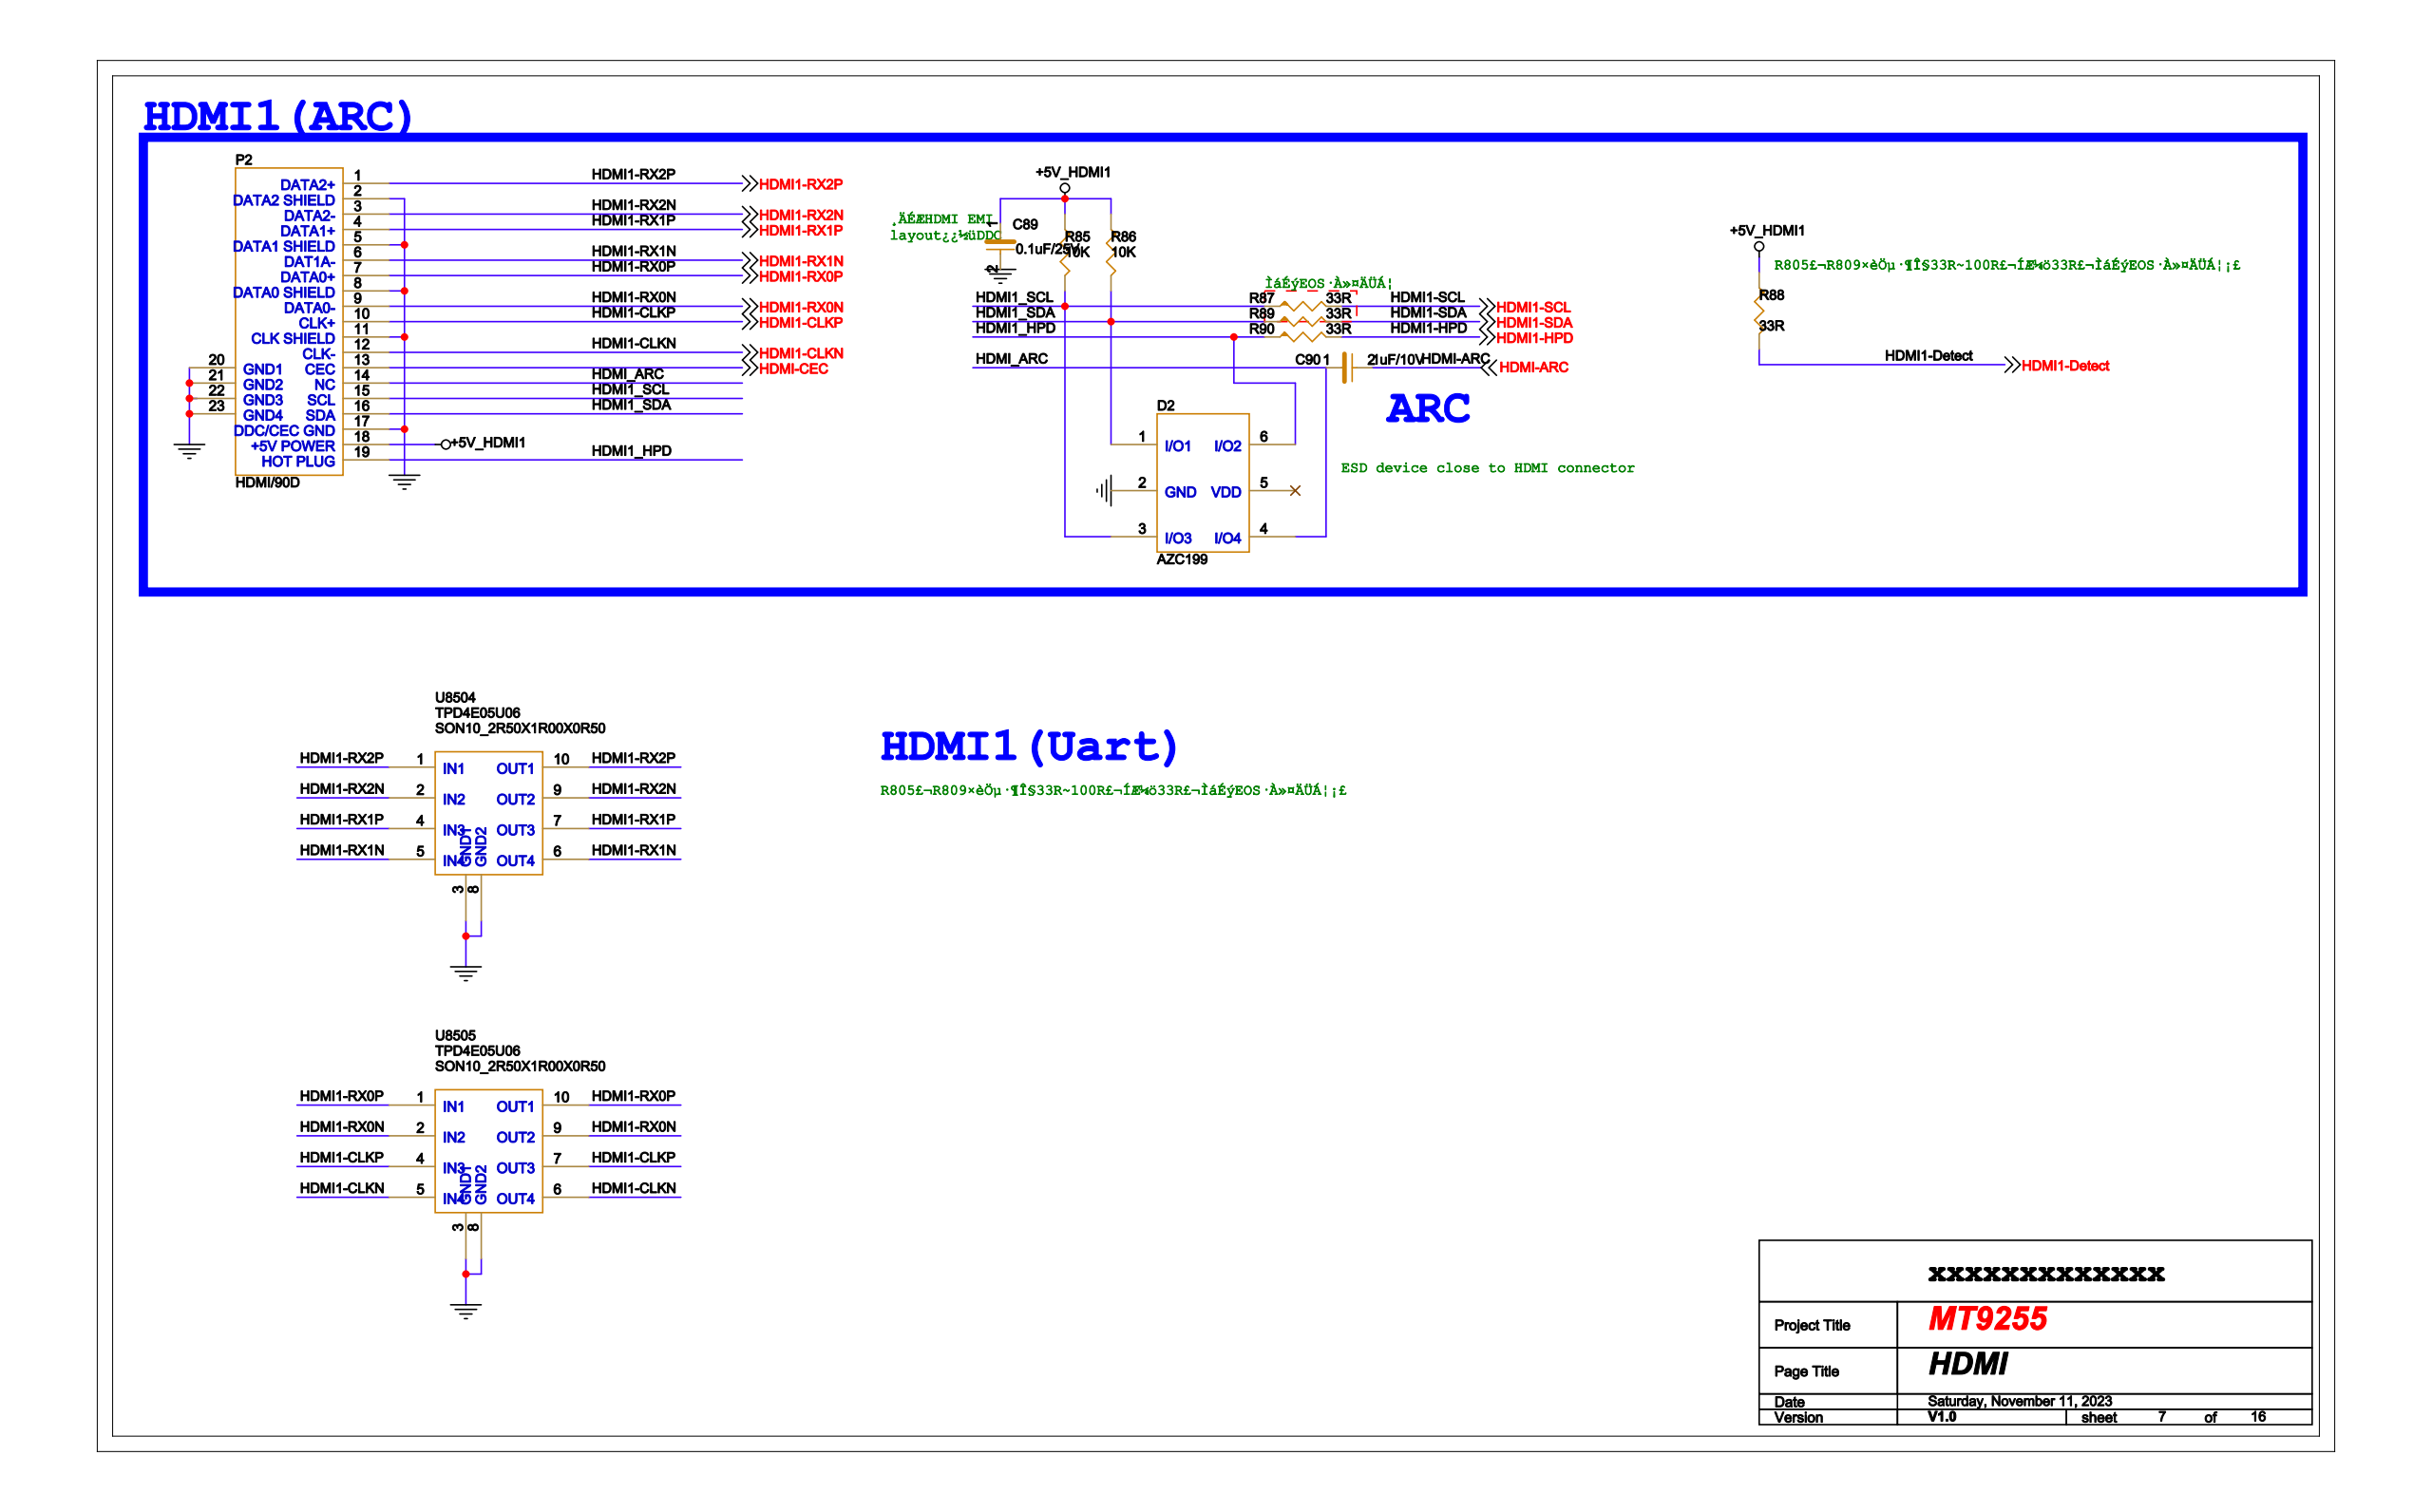Circuit board | Cadence Allegro | 1223 parts | 777 nets | one sheet of the schematic
Parts on this sheet (reference | value | footprint):
C89 | 0.1uF/25V | C0402
C90 | 1uF/10V | C0402
D2 | AZC199 | SOT-23-6L
P2 | HDMI/90D | HDMI_A
R85 | 10K | R0402
R86 | 10K | R0402
R87 | 33R | R0402
R88 | 33R | R0402
R89 | 33R | R0402
R90 | 33R | R0402
U8504 | TPD4E05U06 | SON10_2R50X1R00X0R50
U8505 | TPD4E05U06 | SON10_2R50X1R00X0R50
Nets of these parts (net: part-pin ...):
GND: C89-2 D2-2 U8504-3 U8504-8 U8505-3 U8505-8 P2-2 P2-5 P2-8 P2-11 P2-17 P2-20 P2-21 P2-22 P2-23
+5V_HDMI1: C89-1 R85-1 R86-1 R88-1 P2-18
HDMI_ARC: C90-1 D2-4 P2-14
HDMI-ARC: C90-2
HDMI1_SDA: D2-1 R86-2 R89-1 P2-16
HDMI1_HPD: D2-6 R90-1 P2-19
HDMI1_SCL: D2-3 R85-2 R87-1 P2-15
HDMI-CEC: P2-13
HDMI1-CLKP: U8505-4 U8505-7 P2-10
HDMI1-CLKN: U8505-5 U8505-6 P2-12
HDMI1-RX1N: U8504-5 U8504-6 P2-6
HDMI1-RX0P: U8505-1 U8505-10 P2-7
HDMI1-RX0N: U8505-2 U8505-9 P2-9
HDMI1-RX1P: U8504-4 U8504-7 P2-4
HDMI1-RX2P: U8504-1 U8504-10 P2-1
HDMI1-RX2N: U8504-2 U8504-9 P2-3
HDMI1-SCL: R87-2
HDMI1-DETECT: R88-2
HDMI1-SDA: R89-2
HDMI1-HPD: R90-2